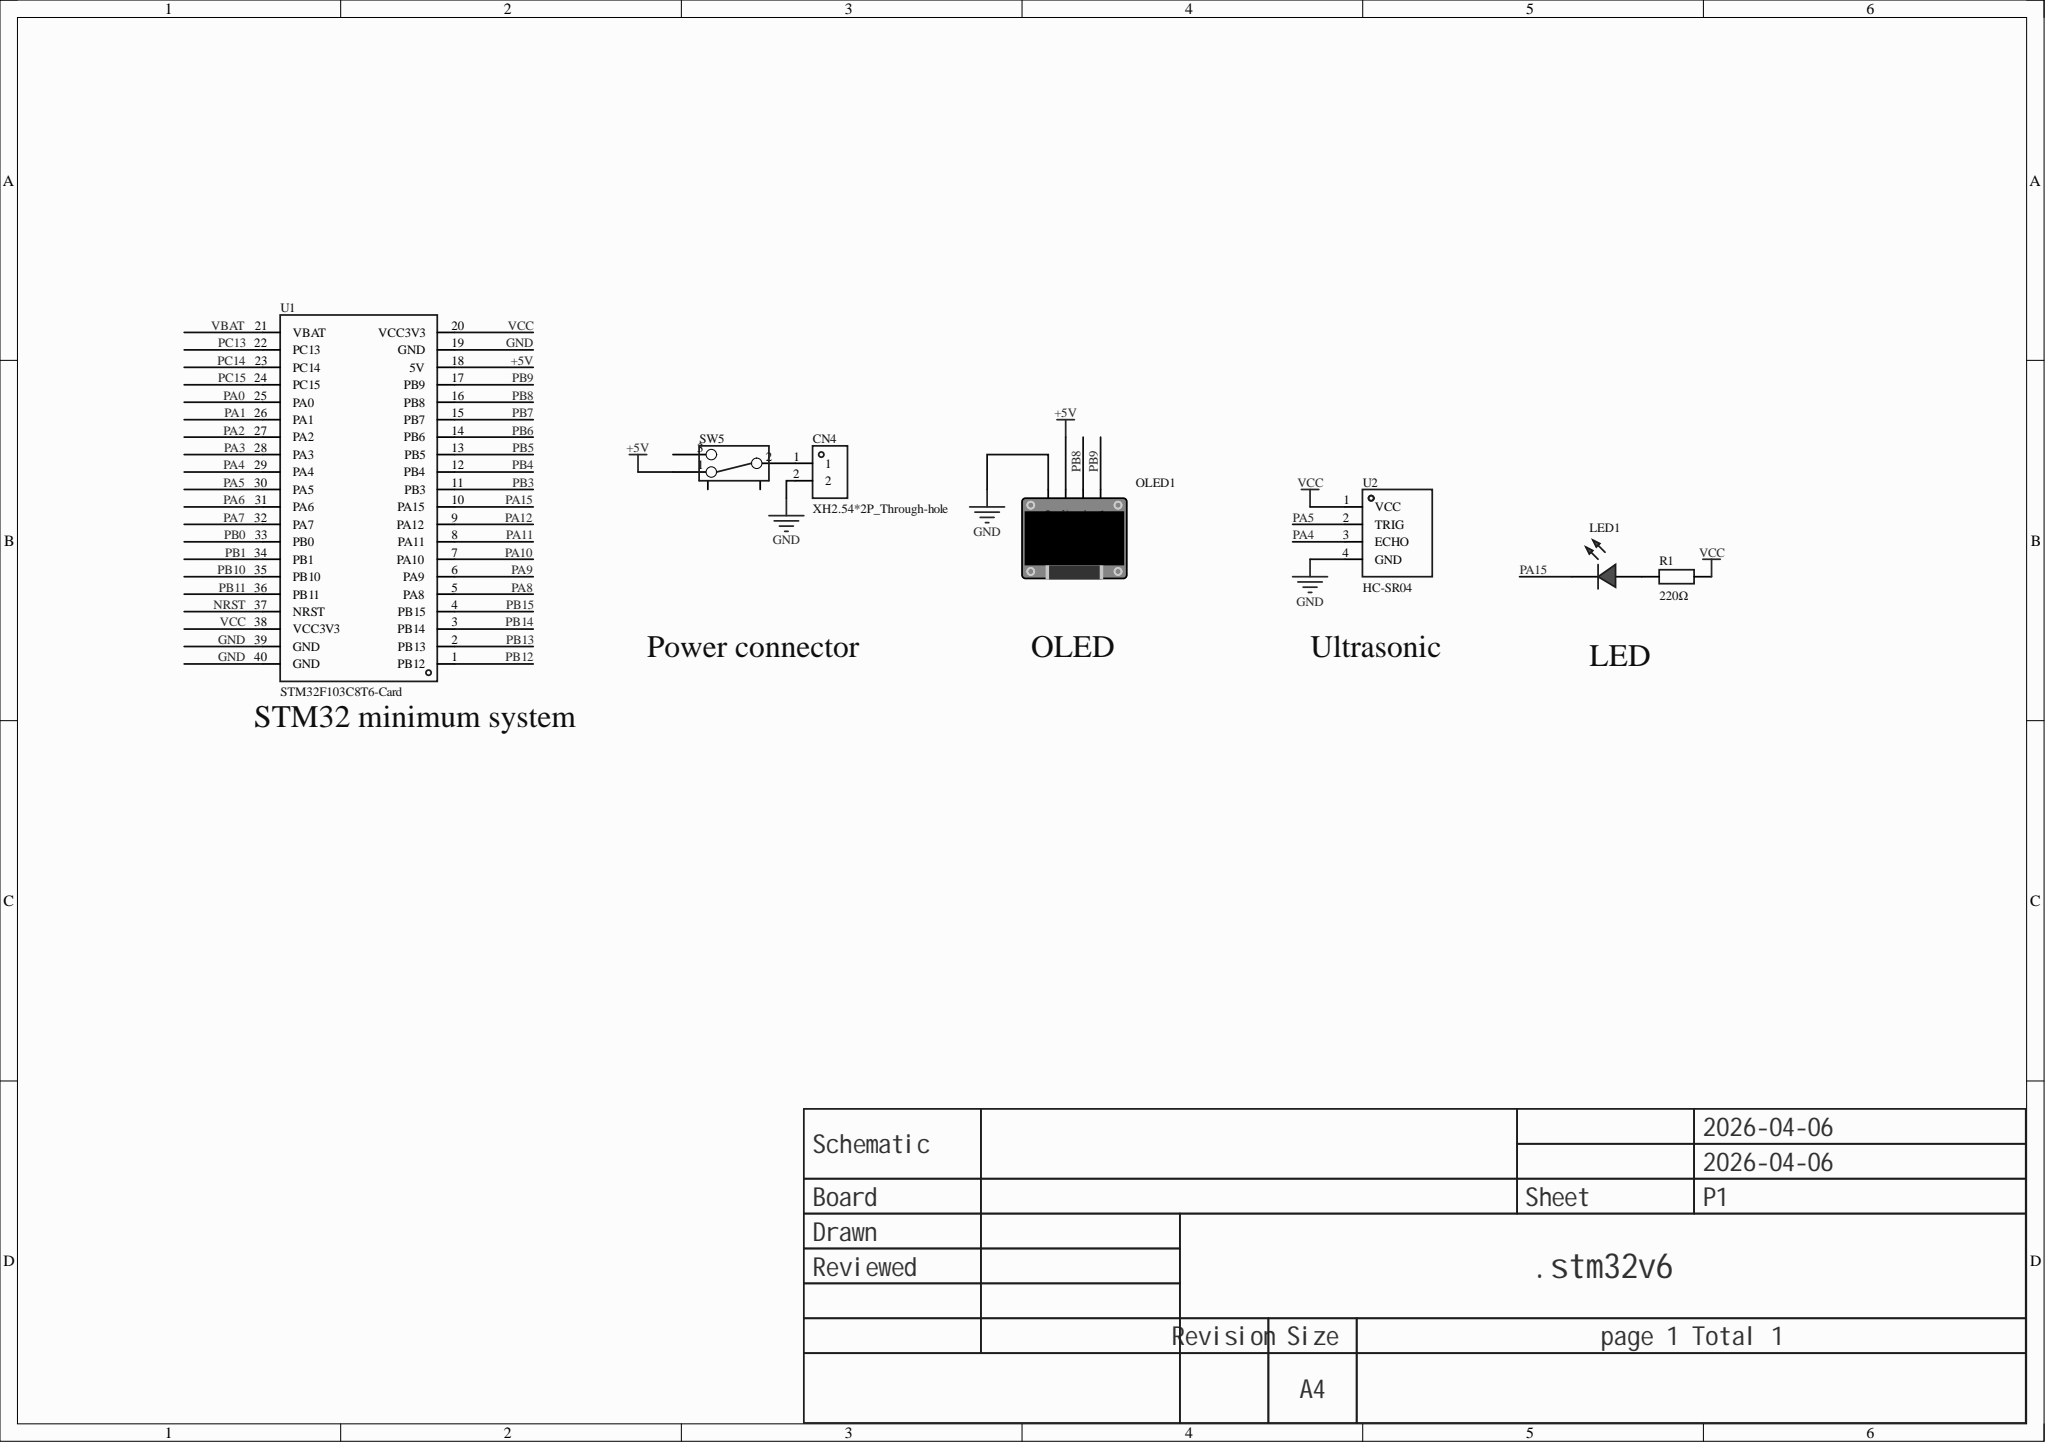Circuit board | Altium Designer | 7 parts | 10 nets
Bill of materials:
Comment,Description,Designator,Footprint,LibRef,Quantity
"XH2.54*2P_Through-hole","","CN4","CONN-TH_2P-P2.50-XH2.54-2P","XH2.54*2P_直插","1"
"","","LED1","LED_TH-3mm","LED_TH-R_3mm","1"
"","","OLED1","0.96OLED_4P","0.96OLED模块_4P","1"
"220Ω","","R1","Res_1/8W","Res_AXIAL-1/8W","1"
"","","SW5","拨动开关","拨动开关_正","1"
"STM32F103C8T6-Card","","U1","CONN-TH_L53.3-W22.9_STM32F103C8T6-CARD","STM32F103C8T6-Card","1"
"HC-SR04","","U2","TH_HC-SR04V","HC-SR04","1"
Netlist (Protel format):
[
CN4
CONN-TH_2P-P2.50-XH2.54-2P
XH2.54*2P_Through-hole



]
[
LED1
LED_TH-3mm




]
[
OLED1
0.96OLED_4P




]
[
R1
Res_1/8W
220Ω



]
[
SW5
拨动开关




]
[
U1
CONN-TH_L53.3-W22.9_STM32F103C8T6-CARD
STM32F103C8T6-Card



]
[
U2
TH_HC-SR04V
HC-SR04



]
(
VCC
R1-2
U1-20
U1-38
U2-1
)
(
PB9
OLED1-4
U1-17
)
(
PB8
OLED1-3
U1-16
)
(
PA15
LED1-2
U1-10
)
(
PA5
U1-30
U2-2
)
(
PA4
U1-29
U2-3
)
(
NetLED1_1
LED1-1
R1-1
)
(
NetCN4_1
CN4-1
SW5-2
)
(
GND
CN4-2
OLED1-1
U1-19
U1-39
U1-40
U2-4
)
(
+5V
OLED1-2
SW5-1
U1-18
)